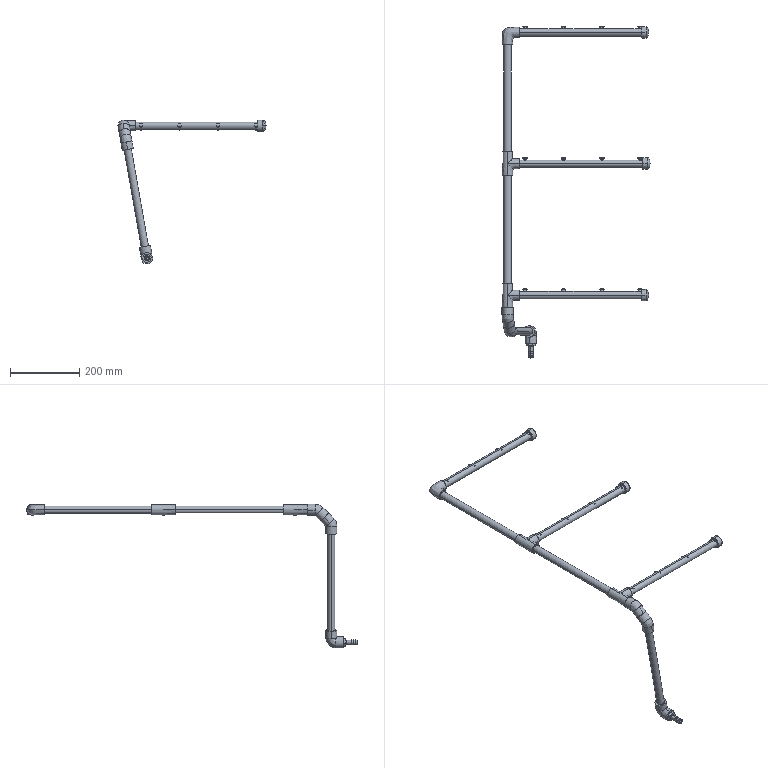Part | SolidWorks | 30 solids | 667 faces | box 428.236 x 959.541 x 415.929 mm | volume 725638 mm3 | cylinder 260 | cone 166 | plane 160 | torus 46 | spline 35 | commonest cylinder face diameters 8 x48 6.476 x24 10 x24 10.8 x24 10.935 x24 12.15 x24